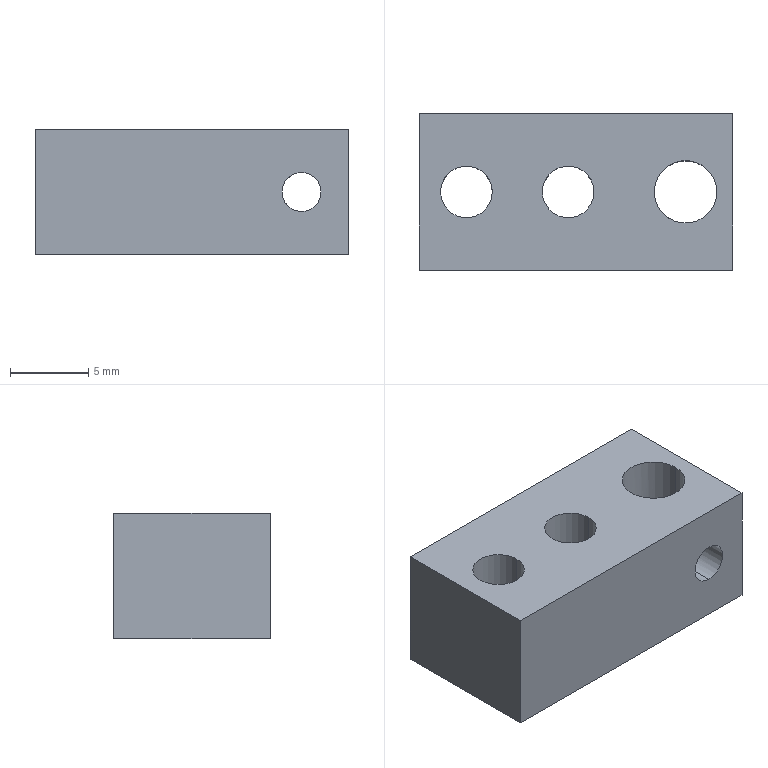Part | SolidWorks | features HoleWzd 2, Extrusion 1, ICE 1, MoveFace 1 | 1 solid | 16 faces | box 20 x 10 x 8 mm | volume 1332 mm3 | cylinder 10 | plane 6 | commonest cylinder face diameters 2.5 x4 3.3 x4 4 x2
STEP:
#1=CARTESIAN_POINT('',(0.,-5.,2.75));
#2=VERTEX_POINT('',#1);
#3=CARTESIAN_POINT('',(0.,-5.,5.25));
#4=VERTEX_POINT('',#3);
#5=CARTESIAN_POINT('',(0.,-5.,4.));
#6=DIRECTION('',(0.,1.,0.));
#7=DIRECTION('',(0.,0.,1.));
#8=AXIS2_PLACEMENT_3D('',#5,#6,#7);
#9=CIRCLE('',#8,1.25);
#10=EDGE_CURVE('',#2,#4,#9,.T.);
#11=ORIENTED_EDGE('',*,*,#10,.F.);
#12=CARTESIAN_POINT('',(0.,-2.,2.75));
#13=VERTEX_POINT('',#12);
#14=CARTESIAN_POINT('',(0.,5.,2.75));
#15=DIRECTION('',(0.,1.,0.));
#16=VECTOR('',#15,1000.);
#17=LINE('',#14,#16);
#18=EDGE_CURVE('',#2,#13,#17,.T.);
#19=ORIENTED_EDGE('',*,*,#18,.T.);
#20=CARTESIAN_POINT('',(0.,-2.,5.25));
#21=VERTEX_POINT('',#20);
#22=CARTESIAN_POINT('',(0.,-2.,2.75));
#23=CARTESIAN_POINT('',(-0.1686,-2.,2.75));
#24=CARTESIAN_POINT('',(-0.3364,-1.978,2.785));
#25=CARTESIAN_POINT('',(-0.6379,-1.902,2.913));
#26=CARTESIAN_POINT('',(-0.773,-1.849,3.005));
#27=CARTESIAN_POINT('',(-0.9982,-1.738,3.231));
#28=CARTESIAN_POINT('',(-1.088,-1.68,3.363));
#29=CARTESIAN_POINT('',(-1.183,-1.613,3.589));
#30=CARTESIAN_POINT('',(-1.208,-1.594,3.667));
#31=CARTESIAN_POINT('',(-1.241,-1.568,3.83));
#32=CARTESIAN_POINT('',(-1.25,-1.561,3.916));
#33=CARTESIAN_POINT('',(-1.25,-1.561,4.167));
#34=CARTESIAN_POINT('',(-1.215,-1.59,4.335));
#35=CARTESIAN_POINT('',(-1.089,-1.679,4.635));
#36=CARTESIAN_POINT('',(-0.9979,-1.738,4.769));
#37=CARTESIAN_POINT('',(-0.8293,-1.821,4.939));
#38=CARTESIAN_POINT('',(-0.7682,-1.848,4.989));
#39=CARTESIAN_POINT('',(-0.6354,-1.898,5.079));
#40=CARTESIAN_POINT('',(-0.5628,-1.921,5.119));
#41=CARTESIAN_POINT('',(-0.4124,-1.959,5.183));
#42=CARTESIAN_POINT('',(-0.3341,-1.974,5.207));
#43=CARTESIAN_POINT('',(-0.1706,-1.994,5.241));
#44=CARTESIAN_POINT('',(-0.08492,-2.,5.25));
#45=CARTESIAN_POINT('',(0.,-2.,5.25));
#46=B_SPLINE_CURVE_WITH_KNOTS('',3,(#22,#23,#24,#25,#26,#27,#28,#29,#30,#31,#32,#33,#34,#35,#36,#37,#38,#39,#40,#41,#42,#43,#44,#45),.UNSPECIFIED.,.F.,.F.,(4,2,2,2,2,2,2,2,2,2,2,4),(0.004021,0.004522,0.005024,0.005525,0.005776,0.006027,0.006528,0.00703,0.007281,0.007531,0.007782,0.008033),.UNSPECIFIED.);
#47=EDGE_CURVE('',#13,#21,#46,.T.);
#48=ORIENTED_EDGE('',*,*,#47,.T.);
#49=CARTESIAN_POINT('',(0.,5.,5.25));
#50=DIRECTION('',(0.,1.,0.));
#51=VECTOR('',#50,1000.);
#52=LINE('',#49,#51);
#53=EDGE_CURVE('',#4,#21,#52,.T.);
#54=ORIENTED_EDGE('',*,*,#53,.F.);
#55=EDGE_LOOP('',(#11,#19,#48,#54));
#56=FACE_OUTER_BOUND('',#55,.T.);
#57=CARTESIAN_POINT('',(0.,5.,4.));
#58=DIRECTION('',(0.,1.,0.));
#59=DIRECTION('',(0.,0.,1.));
#60=AXIS2_PLACEMENT_3D('',#57,#58,#59);
#61=CYLINDRICAL_SURFACE('',#60,1.25);
#62=ADVANCED_FACE('',(#56),#61,.F.);
#63=CARTESIAN_POINT('',(0.,2.,5.25));
#64=VERTEX_POINT('',#63);
#65=CARTESIAN_POINT('',(0.,2.,2.75));
#66=VERTEX_POINT('',#65);
#67=CARTESIAN_POINT('',(0.,2.,5.25));
#68=CARTESIAN_POINT('',(-0.08511,2.,5.25));
#69=CARTESIAN_POINT('',(-0.1684,1.995,5.241));
#70=CARTESIAN_POINT('',(-0.3316,1.974,5.208));
#71=CARTESIAN_POINT('',(-0.4122,1.959,5.183));
#72=CARTESIAN_POINT('',(-0.6385,1.902,5.087));
#73=CARTESIAN_POINT('',(-0.7738,1.848,4.994));
#74=CARTESIAN_POINT('',(-0.9977,1.738,4.77));
#75=CARTESIAN_POINT('',(-1.088,1.68,4.636));
#76=CARTESIAN_POINT('',(-1.214,1.591,4.338));
#77=CARTESIAN_POINT('',(-1.25,1.561,4.17));
#78=CARTESIAN_POINT('',(-1.25,1.561,3.831));
#79=CARTESIAN_POINT('',(-1.215,1.591,3.664));
#80=CARTESIAN_POINT('',(-1.089,1.68,3.365));
#81=CARTESIAN_POINT('',(-0.9982,1.738,3.231));
#82=CARTESIAN_POINT('',(-0.7723,1.849,3.004));
#83=CARTESIAN_POINT('',(-0.6398,1.901,2.913));
#84=CARTESIAN_POINT('',(-0.4108,1.959,2.817));
#85=CARTESIAN_POINT('',(-0.332,1.974,2.792));
#86=CARTESIAN_POINT('',(-0.1695,1.994,2.759));
#87=CARTESIAN_POINT('',(-0.0845,2.,2.75));
#88=CARTESIAN_POINT('',(0.,2.,2.75));
#89=B_SPLINE_CURVE_WITH_KNOTS('',3,(#67,#68,#69,#70,#71,#72,#73,#74,#75,#76,#77,#78,#79,#80,#81,#82,#83,#84,#85,#86,#87,#88),.UNSPECIFIED.,.F.,.F.,(4,2,2,2,2,2,2,2,2,2,4),(0.,0.0002513,0.0005026,0.001005,0.001508,0.002011,0.002513,0.003016,0.003518,0.00377,0.004021),.UNSPECIFIED.);
#90=EDGE_CURVE('',#64,#66,#89,.T.);
#91=ORIENTED_EDGE('',*,*,#90,.T.);
#92=CARTESIAN_POINT('',(0.,5.,2.75));
#93=VERTEX_POINT('',#92);
#94=CARTESIAN_POINT('',(0.,5.,2.75));
#95=DIRECTION('',(0.,1.,0.));
#96=VECTOR('',#95,1000.);
#97=LINE('',#94,#96);
#98=EDGE_CURVE('',#66,#93,#97,.T.);
#99=ORIENTED_EDGE('',*,*,#98,.T.);
#100=CARTESIAN_POINT('',(0.,5.,5.25));
#101=VERTEX_POINT('',#100);
#102=CARTESIAN_POINT('',(0.,5.,4.));
#103=DIRECTION('',(0.,1.,0.));
#104=DIRECTION('',(0.,0.,1.));
#105=AXIS2_PLACEMENT_3D('',#102,#103,#104);
#106=CIRCLE('',#105,1.25);
#107=EDGE_CURVE('',#93,#101,#106,.T.);
#108=ORIENTED_EDGE('',*,*,#107,.T.);
#109=CARTESIAN_POINT('',(0.,5.,5.25));
#110=DIRECTION('',(0.,1.,0.));
#111=VECTOR('',#110,1000.);
#112=LINE('',#109,#111);
#113=EDGE_CURVE('',#64,#101,#112,.T.);
#114=ORIENTED_EDGE('',*,*,#113,.F.);
#115=EDGE_LOOP('',(#91,#99,#108,#114));
#116=FACE_OUTER_BOUND('',#115,.T.);
#117=CARTESIAN_POINT('',(0.,5.,4.));
#118=DIRECTION('',(0.,1.,0.));
#119=DIRECTION('',(0.,0.,1.));
#120=AXIS2_PLACEMENT_3D('',#117,#118,#119);
#121=CYLINDRICAL_SURFACE('',#120,1.25);
#122=ADVANCED_FACE('',(#116),#121,.F.);
#123=CARTESIAN_POINT('',(-9.15,0.,8.));
#124=VERTEX_POINT('',#123);
#125=CARTESIAN_POINT('',(-5.85,0.,8.));
#126=VERTEX_POINT('',#125);
#127=CARTESIAN_POINT('',(-7.5,0.,8.));
#128=DIRECTION('',(0.,0.,1.));
#129=DIRECTION('',(1.,0.,0.));
#130=AXIS2_PLACEMENT_3D('',#127,#128,#129);
#131=CIRCLE('',#130,1.65);
#132=EDGE_CURVE('',#124,#126,#131,.T.);
#133=ORIENTED_EDGE('',*,*,#132,.T.);
#134=CARTESIAN_POINT('',(-5.85,0.,0.));
#135=VERTEX_POINT('',#134);
#136=CARTESIAN_POINT('',(-5.85,0.,0.));
#137=DIRECTION('',(0.,0.,-1.));
#138=VECTOR('',#137,1000.);
#139=LINE('',#136,#138);
#140=EDGE_CURVE('',#126,#135,#139,.T.);
#141=ORIENTED_EDGE('',*,*,#140,.T.);
#142=CARTESIAN_POINT('',(-9.15,0.,0.));
#143=VERTEX_POINT('',#142);
#144=CARTESIAN_POINT('',(-7.5,0.,0.));
#145=DIRECTION('',(0.,0.,-1.));
#146=DIRECTION('',(-1.,0.,0.));
#147=AXIS2_PLACEMENT_3D('',#144,#145,#146);
#148=CIRCLE('',#147,1.65);
#149=EDGE_CURVE('',#135,#143,#148,.T.);
#150=ORIENTED_EDGE('',*,*,#149,.T.);
#151=CARTESIAN_POINT('',(-9.15,0.,0.));
#152=DIRECTION('',(0.,0.,-1.));
#153=VECTOR('',#152,1000.);
#154=LINE('',#151,#153);
#155=EDGE_CURVE('',#124,#143,#154,.T.);
#156=ORIENTED_EDGE('',*,*,#155,.F.);
#157=EDGE_LOOP('',(#133,#141,#150,#156));
#158=FACE_OUTER_BOUND('',#157,.T.);
#159=CARTESIAN_POINT('',(-7.5,0.,0.));
#160=DIRECTION('',(0.,0.,-1.));
#161=DIRECTION('',(-1.,0.,0.));
#162=AXIS2_PLACEMENT_3D('',#159,#160,#161);
#163=CYLINDRICAL_SURFACE('',#162,1.65);
#164=ADVANCED_FACE('',(#158),#163,.F.);
#165=CARTESIAN_POINT('',(-15.65,0.,8.));
#166=VERTEX_POINT('',#165);
#167=CARTESIAN_POINT('',(-12.35,0.,8.));
#168=VERTEX_POINT('',#167);
#169=CARTESIAN_POINT('',(-14.,0.,8.));
#170=DIRECTION('',(0.,0.,1.));
#171=DIRECTION('',(1.,0.,0.));
#172=AXIS2_PLACEMENT_3D('',#169,#170,#171);
#173=CIRCLE('',#172,1.65);
#174=EDGE_CURVE('',#166,#168,#173,.T.);
#175=ORIENTED_EDGE('',*,*,#174,.T.);
#176=CARTESIAN_POINT('',(-12.35,0.,0.));
#177=VERTEX_POINT('',#176);
#178=CARTESIAN_POINT('',(-12.35,0.,0.));
#179=DIRECTION('',(0.,0.,-1.));
#180=VECTOR('',#179,1000.);
#181=LINE('',#178,#180);
#182=EDGE_CURVE('',#168,#177,#181,.T.);
#183=ORIENTED_EDGE('',*,*,#182,.T.);
#184=CARTESIAN_POINT('',(-15.65,0.,0.));
#185=VERTEX_POINT('',#184);
#186=CARTESIAN_POINT('',(-14.,0.,0.));
#187=DIRECTION('',(0.,0.,-1.));
#188=DIRECTION('',(-1.,0.,0.));
#189=AXIS2_PLACEMENT_3D('',#186,#187,#188);
#190=CIRCLE('',#189,1.65);
#191=EDGE_CURVE('',#177,#185,#190,.T.);
#192=ORIENTED_EDGE('',*,*,#191,.T.);
#193=CARTESIAN_POINT('',(-15.65,0.,0.));
#194=DIRECTION('',(0.,0.,-1.));
#195=VECTOR('',#194,1000.);
#196=LINE('',#193,#195);
#197=EDGE_CURVE('',#166,#185,#196,.T.);
#198=ORIENTED_EDGE('',*,*,#197,.F.);
#199=EDGE_LOOP('',(#175,#183,#192,#198));
#200=FACE_OUTER_BOUND('',#199,.T.);
#201=CARTESIAN_POINT('',(-14.,0.,0.));
#202=DIRECTION('',(0.,0.,-1.));
#203=DIRECTION('',(-1.,0.,0.));
#204=AXIS2_PLACEMENT_3D('',#201,#202,#203);
#205=CYLINDRICAL_SURFACE('',#204,1.65);
#206=ADVANCED_FACE('',(#200),#205,.F.);
#207=CARTESIAN_POINT('',(0.,-2.,5.25));
#208=CARTESIAN_POINT('',(0.08511,-2.,5.25));
#209=CARTESIAN_POINT('',(0.1684,-1.995,5.241));
#210=CARTESIAN_POINT('',(0.3316,-1.974,5.208));
#211=CARTESIAN_POINT('',(0.4122,-1.959,5.183));
#212=CARTESIAN_POINT('',(0.6385,-1.902,5.087));
#213=CARTESIAN_POINT('',(0.7738,-1.848,4.994));
#214=CARTESIAN_POINT('',(0.9977,-1.738,4.77));
#215=CARTESIAN_POINT('',(1.088,-1.68,4.636));
#216=CARTESIAN_POINT('',(1.214,-1.591,4.338));
#217=CARTESIAN_POINT('',(1.25,-1.561,4.17));
#218=CARTESIAN_POINT('',(1.25,-1.561,3.831));
#219=CARTESIAN_POINT('',(1.215,-1.591,3.664));
#220=CARTESIAN_POINT('',(1.089,-1.68,3.365));
#221=CARTESIAN_POINT('',(0.9982,-1.738,3.231));
#222=CARTESIAN_POINT('',(0.7723,-1.849,3.004));
#223=CARTESIAN_POINT('',(0.6398,-1.901,2.913));
#224=CARTESIAN_POINT('',(0.4108,-1.959,2.817));
#225=CARTESIAN_POINT('',(0.332,-1.974,2.792));
#226=CARTESIAN_POINT('',(0.1695,-1.994,2.759));
#227=CARTESIAN_POINT('',(0.0845,-2.,2.75));
#228=CARTESIAN_POINT('',(0.,-2.,2.75));
#229=B_SPLINE_CURVE_WITH_KNOTS('',3,(#207,#208,#209,#210,#211,#212,#213,#214,#215,#216,#217,#218,#219,#220,#221,#222,#223,#224,#225,#226,#227,#228),.UNSPECIFIED.,.F.,.F.,(4,2,2,2,2,2,2,2,2,2,4),(0.,0.0002513,0.0005026,0.001005,0.001508,0.002011,0.002513,0.003016,0.003518,0.00377,0.004021),.UNSPECIFIED.);
#230=EDGE_CURVE('',#21,#13,#229,.T.);
#231=ORIENTED_EDGE('',*,*,#230,.F.);
#232=ORIENTED_EDGE('',*,*,#47,.F.);
#233=EDGE_LOOP('',(#231,#232));
#234=FACE_BOUND('',#233,.T.);
#235=CARTESIAN_POINT('',(-2.,0.,8.));
#236=VERTEX_POINT('',#235);
#237=CARTESIAN_POINT('',(2.,0.,8.));
#238=VERTEX_POINT('',#237);
#239=CARTESIAN_POINT('',(0.,0.,8.));
#240=DIRECTION('',(0.,0.,1.));
#241=DIRECTION('',(1.,0.,0.));
#242=AXIS2_PLACEMENT_3D('',#239,#240,#241);
#243=CIRCLE('',#242,2.);
#244=EDGE_CURVE('',#236,#238,#243,.T.);
#245=ORIENTED_EDGE('',*,*,#244,.T.);
#246=CARTESIAN_POINT('',(2.,0.,0.));
#247=VERTEX_POINT('',#246);
#248=CARTESIAN_POINT('',(2.,0.,8.));
#249=DIRECTION('',(0.,0.,-1.));
#250=VECTOR('',#249,1000.);
#251=LINE('',#248,#250);
#252=EDGE_CURVE('',#238,#247,#251,.T.);
#253=ORIENTED_EDGE('',*,*,#252,.T.);
#254=CARTESIAN_POINT('',(-2.,0.,0.));
#255=VERTEX_POINT('',#254);
#256=CARTESIAN_POINT('',(0.,0.,0.));
#257=DIRECTION('',(0.,0.,1.));
#258=DIRECTION('',(1.,0.,0.));
#259=AXIS2_PLACEMENT_3D('',#256,#257,#258);
#260=CIRCLE('',#259,2.);
#261=EDGE_CURVE('',#255,#247,#260,.T.);
#262=ORIENTED_EDGE('',*,*,#261,.F.);
#263=CARTESIAN_POINT('',(-2.,0.,8.));
#264=DIRECTION('',(0.,0.,-1.));
#265=VECTOR('',#264,1000.);
#266=LINE('',#263,#265);
#267=EDGE_CURVE('',#236,#255,#266,.T.);
#268=ORIENTED_EDGE('',*,*,#267,.F.);
#269=EDGE_LOOP('',(#245,#253,#262,#268));
#270=FACE_OUTER_BOUND('',#269,.T.);
#271=CARTESIAN_POINT('',(0.,0.,8.));
#272=DIRECTION('',(0.,0.,-1.));
#273=DIRECTION('',(-1.,0.,0.));
#274=AXIS2_PLACEMENT_3D('',#271,#272,#273);
#275=CYLINDRICAL_SURFACE('',#274,2.);
#276=ADVANCED_FACE('',(#234,#270),#275,.F.);
#277=ORIENTED_EDGE('',*,*,#132,.F.);
#278=CARTESIAN_POINT('',(-7.5,0.,8.));
#279=DIRECTION('',(0.,0.,1.));
#280=DIRECTION('',(1.,0.,0.));
#281=AXIS2_PLACEMENT_3D('',#278,#279,#280);
#282=CIRCLE('',#281,1.65);
#283=EDGE_CURVE('',#126,#124,#282,.T.);
#284=ORIENTED_EDGE('',*,*,#283,.F.);
#285=EDGE_LOOP('',(#277,#284));
#286=FACE_BOUND('',#285,.T.);
#287=ORIENTED_EDGE('',*,*,#174,.F.);
#288=CARTESIAN_POINT('',(-14.,0.,8.));
#289=DIRECTION('',(0.,0.,1.));
#290=DIRECTION('',(1.,0.,0.));
#291=AXIS2_PLACEMENT_3D('',#288,#289,#290);
#292=CIRCLE('',#291,1.65);
#293=EDGE_CURVE('',#168,#166,#292,.T.);
#294=ORIENTED_EDGE('',*,*,#293,.F.);
#295=EDGE_LOOP('',(#287,#294));
#296=FACE_BOUND('',#295,.T.);
#297=CARTESIAN_POINT('',(3.,5.,8.));
#298=VERTEX_POINT('',#297);
#299=CARTESIAN_POINT('',(3.,-5.,8.));
#300=VERTEX_POINT('',#299);
#301=CARTESIAN_POINT('',(3.,0.,8.));
#302=DIRECTION('',(0.,-1.,0.));
#303=VECTOR('',#302,1000.);
#304=LINE('',#301,#303);
#305=EDGE_CURVE('',#298,#300,#304,.T.);
#306=ORIENTED_EDGE('',*,*,#305,.F.);
#307=CARTESIAN_POINT('',(-17.,5.,8.));
#308=VERTEX_POINT('',#307);
#309=CARTESIAN_POINT('',(-10.,5.,8.));
#310=DIRECTION('',(-1.,0.,0.));
#311=VECTOR('',#310,1000.);
#312=LINE('',#309,#311);
#313=EDGE_CURVE('',#298,#308,#312,.T.);
#314=ORIENTED_EDGE('',*,*,#313,.T.);
#315=CARTESIAN_POINT('',(-17.,-5.,8.));
#316=VERTEX_POINT('',#315);
#317=CARTESIAN_POINT('',(-17.,5.,8.));
#318=DIRECTION('',(0.,-1.,0.));
#319=VECTOR('',#318,1000.);
#320=LINE('',#317,#319);
#321=EDGE_CURVE('',#308,#316,#320,.T.);
#322=ORIENTED_EDGE('',*,*,#321,.T.);
#323=CARTESIAN_POINT('',(-10.,-5.,8.));
#324=DIRECTION('',(1.,0.,0.));
#325=VECTOR('',#324,1000.);
#326=LINE('',#323,#325);
#327=EDGE_CURVE('',#316,#300,#326,.T.);
#328=ORIENTED_EDGE('',*,*,#327,.T.);
#329=EDGE_LOOP('',(#306,#314,#322,#328));
#330=FACE_OUTER_BOUND('',#329,.T.);
#331=ORIENTED_EDGE('',*,*,#244,.F.);
#332=CARTESIAN_POINT('',(0.,0.,8.));
#333=DIRECTION('',(0.,0.,1.));
#334=DIRECTION('',(1.,0.,0.));
#335=AXIS2_PLACEMENT_3D('',#332,#333,#334);
#336=CIRCLE('',#335,2.);
#337=EDGE_CURVE('',#238,#236,#336,.T.);
#338=ORIENTED_EDGE('',*,*,#337,.F.);
#339=EDGE_LOOP('',(#331,#338));
#340=FACE_BOUND('',#339,.T.);
#341=CARTESIAN_POINT('',(0.,0.,8.));
#342=DIRECTION('',(0.,0.,1.));
#343=DIRECTION('',(1.,0.,0.));
#344=AXIS2_PLACEMENT_3D('',#341,#342,#343);
#345=PLANE('',#344);
#346=ADVANCED_FACE('',(#286,#296,#330,#340),#345,.T.);
#347=CARTESIAN_POINT('',(-7.5,0.,0.));
#348=DIRECTION('',(0.,0.,-1.));
#349=DIRECTION('',(-1.,0.,0.));
#350=AXIS2_PLACEMENT_3D('',#347,#348,#349);
#351=CIRCLE('',#350,1.65);
#352=EDGE_CURVE('',#143,#135,#351,.T.);
#353=ORIENTED_EDGE('',*,*,#352,.F.);
#354=ORIENTED_EDGE('',*,*,#149,.F.);
#355=EDGE_LOOP('',(#353,#354));
#356=FACE_BOUND('',#355,.T.);
#357=CARTESIAN_POINT('',(-14.,0.,0.));
#358=DIRECTION('',(0.,0.,-1.));
#359=DIRECTION('',(-1.,0.,0.));
#360=AXIS2_PLACEMENT_3D('',#357,#358,#359);
#361=CIRCLE('',#360,1.65);
#362=EDGE_CURVE('',#185,#177,#361,.T.);
#363=ORIENTED_EDGE('',*,*,#362,.F.);
#364=ORIENTED_EDGE('',*,*,#191,.F.);
#365=EDGE_LOOP('',(#363,#364));
#366=FACE_BOUND('',#365,.T.);
#367=CARTESIAN_POINT('',(3.,5.,0.));
#368=VERTEX_POINT('',#367);
#369=CARTESIAN_POINT('',(-17.,5.,0.));
#370=VERTEX_POINT('',#369);
#371=CARTESIAN_POINT('',(-10.,5.,0.));
#372=DIRECTION('',(-1.,0.,0.));
#373=VECTOR('',#372,1000.);
#374=LINE('',#371,#373);
#375=EDGE_CURVE('',#368,#370,#374,.T.);
#376=ORIENTED_EDGE('',*,*,#375,.F.);
#377=CARTESIAN_POINT('',(3.,-5.,0.));
#378=VERTEX_POINT('',#377);
#379=CARTESIAN_POINT('',(3.,10.325,0.));
#380=DIRECTION('',(0.,1.,0.));
#381=VECTOR('',#380,1000.);
#382=LINE('',#379,#381);
#383=EDGE_CURVE('',#378,#368,#382,.T.);
#384=ORIENTED_EDGE('',*,*,#383,.F.);
#385=CARTESIAN_POINT('',(-17.,-5.,0.));
#386=VERTEX_POINT('',#385);
#387=CARTESIAN_POINT('',(-10.,-5.,0.));
#388=DIRECTION('',(1.,0.,0.));
#389=VECTOR('',#388,1000.);
#390=LINE('',#387,#389);
#391=EDGE_CURVE('',#386,#378,#390,.T.);
#392=ORIENTED_EDGE('',*,*,#391,.F.);
#393=CARTESIAN_POINT('',(-17.,5.,0.));
#394=DIRECTION('',(0.,-1.,0.));
#395=VECTOR('',#394,1000.);
#396=LINE('',#393,#395);
#397=EDGE_CURVE('',#370,#386,#396,.T.);
#398=ORIENTED_EDGE('',*,*,#397,.F.);
#399=EDGE_LOOP('',(#376,#384,#392,#398));
#400=FACE_OUTER_BOUND('',#399,.T.);
#401=ORIENTED_EDGE('',*,*,#261,.T.);
#402=CARTESIAN_POINT('',(0.,0.,0.));
#403=DIRECTION('',(0.,0.,1.));
#404=DIRECTION('',(1.,0.,0.));
#405=AXIS2_PLACEMENT_3D('',#402,#403,#404);
#406=CIRCLE('',#405,2.);
#407=EDGE_CURVE('',#247,#255,#406,.T.);
#408=ORIENTED_EDGE('',*,*,#407,.T.);
#409=EDGE_LOOP('',(#401,#408));
#410=FACE_BOUND('',#409,.T.);
#411=CARTESIAN_POINT('',(0.,0.,0.));
#412=DIRECTION('',(0.,0.,1.));
#413=DIRECTION('',(1.,0.,0.));
#414=AXIS2_PLACEMENT_3D('',#411,#412,#413);
#415=PLANE('',#414);
#416=ADVANCED_FACE('',(#356,#366,#400,#410),#415,.F.);
#417=CARTESIAN_POINT('',(0.,5.,4.));
#418=DIRECTION('',(0.,1.,0.));
#419=DIRECTION('',(0.,0.,1.));
#420=AXIS2_PLACEMENT_3D('',#417,#418,#419);
#421=CIRCLE('',#420,1.25);
#422=EDGE_CURVE('',#101,#93,#421,.T.);
#423=ORIENTED_EDGE('',*,*,#422,.F.);
#424=ORIENTED_EDGE('',*,*,#107,.F.);
#425=EDGE_LOOP('',(#423,#424));
#426=FACE_BOUND('',#425,.T.);
#427=ORIENTED_EDGE('',*,*,#313,.F.);
#428=CARTESIAN_POINT('',(3.,5.,8.));
#429=DIRECTION('',(0.,0.,-1.));
#430=VECTOR('',#429,1000.);
#431=LINE('',#428,#430);
#432=EDGE_CURVE('',#298,#368,#431,.T.);
#433=ORIENTED_EDGE('',*,*,#432,.T.);
#434=ORIENTED_EDGE('',*,*,#375,.T.);
#435=CARTESIAN_POINT('',(-17.,5.,8.));
#436=DIRECTION('',(0.,0.,-1.));
#437=VECTOR('',#436,1000.);
#438=LINE('',#435,#437);
#439=EDGE_CURVE('',#308,#370,#438,.T.);
#440=ORIENTED_EDGE('',*,*,#439,.F.);
#441=EDGE_LOOP('',(#427,#433,#434,#440));
#442=FACE_OUTER_BOUND('',#441,.T.);
#443=CARTESIAN_POINT('',(-10.,5.,8.));
#444=DIRECTION('',(0.,-1.,0.));
#445=DIRECTION('',(0.,0.,-1.));
#446=AXIS2_PLACEMENT_3D('',#443,#444,#445);
#447=PLANE('',#446);
#448=ADVANCED_FACE('',(#426,#442),#447,.F.);
#449=ORIENTED_EDGE('',*,*,#397,.T.);
#450=CARTESIAN_POINT('',(-17.,-5.,8.));
#451=DIRECTION('',(0.,0.,-1.));
#452=VECTOR('',#451,1000.);
#453=LINE('',#450,#452);
#454=EDGE_CURVE('',#316,#386,#453,.T.);
#455=ORIENTED_EDGE('',*,*,#454,.F.);
#456=ORIENTED_EDGE('',*,*,#321,.F.);
#457=ORIENTED_EDGE('',*,*,#439,.T.);
#458=EDGE_LOOP('',(#449,#455,#456,#457));
#459=FACE_OUTER_BOUND('',#458,.T.);
#460=CARTESIAN_POINT('',(-17.,5.,8.));
#461=DIRECTION('',(1.,0.,0.));
#462=DIRECTION('',(0.,1.,0.));
#463=AXIS2_PLACEMENT_3D('',#460,#461,#462);
#464=PLANE('',#463);
#465=ADVANCED_FACE('',(#459),#464,.F.);
#466=CARTESIAN_POINT('',(0.,-5.,4.));
#467=DIRECTION('',(0.,1.,0.));
#468=DIRECTION('',(0.,0.,1.));
#469=AXIS2_PLACEMENT_3D('',#466,#467,#468);
#470=CIRCLE('',#469,1.25);
#471=EDGE_CURVE('',#4,#2,#470,.T.);
#472=ORIENTED_EDGE('',*,*,#471,.T.);
#473=ORIENTED_EDGE('',*,*,#10,.T.);
#474=EDGE_LOOP('',(#472,#473));
#475=FACE_BOUND('',#474,.T.);
#476=ORIENTED_EDGE('',*,*,#391,.T.);
#477=CARTESIAN_POINT('',(3.,-5.,8.));
#478=DIRECTION('',(0.,0.,1.));
#479=VECTOR('',#478,1000.);
#480=LINE('',#477,#479);
#481=EDGE_CURVE('',#378,#300,#480,.T.);
#482=ORIENTED_EDGE('',*,*,#481,.T.);
#483=ORIENTED_EDGE('',*,*,#327,.F.);
#484=ORIENTED_EDGE('',*,*,#454,.T.);
#485=EDGE_LOOP('',(#476,#482,#483,#484));
#486=FACE_OUTER_BOUND('',#485,.T.);
#487=CARTESIAN_POINT('',(-10.,-5.,8.));
#488=DIRECTION('',(0.,1.,0.));
#489=DIRECTION('',(0.,0.,1.));
#490=AXIS2_PLACEMENT_3D('',#487,#488,#489);
#491=PLANE('',#490);
#492=ADVANCED_FACE('',(#475,#486),#491,.F.);
#493=ORIENTED_EDGE('',*,*,#252,.F.);
#494=ORIENTED_EDGE('',*,*,#337,.T.);
#495=ORIENTED_EDGE('',*,*,#267,.T.);
#496=ORIENTED_EDGE('',*,*,#407,.F.);
#497=EDGE_LOOP('',(#493,#494,#495,#496));
#498=FACE_OUTER_BOUND('',#497,.T.);
#499=ORIENTED_EDGE('',*,*,#90,.F.);
#500=CARTESIAN_POINT('',(0.,2.,2.75));
#501=CARTESIAN_POINT('',(0.1686,2.,2.75));
#502=CARTESIAN_POINT('',(0.3364,1.978,2.785));
#503=CARTESIAN_POINT('',(0.6379,1.902,2.913));
#504=CARTESIAN_POINT('',(0.773,1.849,3.005));
#505=CARTESIAN_POINT('',(0.9982,1.738,3.231));
#506=CARTESIAN_POINT('',(1.088,1.68,3.363));
#507=CARTESIAN_POINT('',(1.183,1.613,3.589));
#508=CARTESIAN_POINT('',(1.208,1.594,3.667));
#509=CARTESIAN_POINT('',(1.241,1.568,3.83));
#510=CARTESIAN_POINT('',(1.25,1.561,3.916));
#511=CARTESIAN_POINT('',(1.25,1.561,4.167));
#512=CARTESIAN_POINT('',(1.215,1.59,4.335));
#513=CARTESIAN_POINT('',(1.089,1.679,4.635));
#514=CARTESIAN_POINT('',(0.9979,1.738,4.769));
#515=CARTESIAN_POINT('',(0.8293,1.821,4.939));
#516=CARTESIAN_POINT('',(0.7682,1.848,4.989));
#517=CARTESIAN_POINT('',(0.6354,1.898,5.079));
#518=CARTESIAN_POINT('',(0.5628,1.921,5.119));
#519=CARTESIAN_POINT('',(0.4124,1.959,5.183));
#520=CARTESIAN_POINT('',(0.3341,1.974,5.207));
#521=CARTESIAN_POINT('',(0.1706,1.994,5.241));
#522=CARTESIAN_POINT('',(0.08492,2.,5.25));
#523=CARTESIAN_POINT('',(0.,2.,5.25));
#524=B_SPLINE_CURVE_WITH_KNOTS('',3,(#500,#501,#502,#503,#504,#505,#506,#507,#508,#509,#510,#511,#512,#513,#514,#515,#516,#517,#518,#519,#520,#521,#522,#523),.UNSPECIFIED.,.F.,.F.,(4,2,2,2,2,2,2,2,2,2,2,4),(0.004021,0.004522,0.005024,0.005525,0.005776,0.006027,0.006528,0.00703,0.007281,0.007531,0.007782,0.008033),.UNSPECIFIED.);
#525=EDGE_CURVE('',#66,#64,#524,.T.);
#526=ORIENTED_EDGE('',*,*,#525,.F.);
#527=EDGE_LOOP('',(#499,#526));
#528=FACE_BOUND('',#527,.T.);
#529=CARTESIAN_POINT('',(0.,0.,8.));
#530=DIRECTION('',(0.,0.,-1.));
#531=DIRECTION('',(-1.,0.,0.));
#532=AXIS2_PLACEMENT_3D('',#529,#530,#531);
#533=CYLINDRICAL_SURFACE('',#532,2.);
#534=ADVANCED_FACE('',(#498,#528),#533,.F.);
#535=ORIENTED_EDGE('',*,*,#305,.T.);
#536=ORIENTED_EDGE('',*,*,#481,.F.);
#537=ORIENTED_EDGE('',*,*,#383,.T.);
#538=ORIENTED_EDGE('',*,*,#432,.F.);
#539=EDGE_LOOP('',(#535,#536,#537,#538));
#540=FACE_OUTER_BOUND('',#539,.T.);
#541=CARTESIAN_POINT('',(3.,10.325,22.));
#542=DIRECTION('',(-1.,0.,0.));
#543=DIRECTION('',(0.,-1.,0.));
#544=AXIS2_PLACEMENT_3D('',#541,#542,#543);
#545=PLANE('',#544);
#546=ADVANCED_FACE('',(#540),#545,.F.);
#547=ORIENTED_EDGE('',*,*,#182,.F.);
#548=ORIENTED_EDGE('',*,*,#293,.T.);
#549=ORIENTED_EDGE('',*,*,#197,.T.);
#550=ORIENTED_EDGE('',*,*,#362,.T.);
#551=EDGE_LOOP('',(#547,#548,#549,#550));
#552=FACE_OUTER_BOUND('',#551,.T.);
#553=CARTESIAN_POINT('',(-14.,0.,0.));
#554=DIRECTION('',(0.,0.,-1.));
#555=DIRECTION('',(-1.,0.,0.));
#556=AXIS2_PLACEMENT_3D('',#553,#554,#555);
#557=CYLINDRICAL_SURFACE('',#556,1.65);
#558=ADVANCED_FACE('',(#552),#557,.F.);
#559=ORIENTED_EDGE('',*,*,#140,.F.);
#560=ORIENTED_EDGE('',*,*,#283,.T.);
#561=ORIENTED_EDGE('',*,*,#155,.T.);
#562=ORIENTED_EDGE('',*,*,#352,.T.);
#563=EDGE_LOOP('',(#559,#560,#561,#562));
#564=FACE_OUTER_BOUND('',#563,.T.);
#565=CARTESIAN_POINT('',(-7.5,0.,0.));
#566=DIRECTION('',(0.,0.,-1.));
#567=DIRECTION('',(-1.,0.,0.));
#568=AXIS2_PLACEMENT_3D('',#565,#566,#567);
#569=CYLINDRICAL_SURFACE('',#568,1.65);
#570=ADVANCED_FACE('',(#564),#569,.F.);
#571=ORIENTED_EDGE('',*,*,#98,.F.);
#572=ORIENTED_EDGE('',*,*,#525,.T.);
#573=ORIENTED_EDGE('',*,*,#113,.T.);
#574=ORIENTED_EDGE('',*,*,#422,.T.);
#575=EDGE_LOOP('',(#571,#572,#573,#574));
#576=FACE_OUTER_BOUND('',#575,.T.);
#577=CARTESIAN_POINT('',(0.,5.,4.));
#578=DIRECTION('',(0.,1.,0.));
#579=DIRECTION('',(0.,0.,1.));
#580=AXIS2_PLACEMENT_3D('',#577,#578,#579);
#581=CYLINDRICAL_SURFACE('',#580,1.25);
#582=ADVANCED_FACE('',(#576),#581,.F.);
#583=ORIENTED_EDGE('',*,*,#18,.F.);
#584=ORIENTED_EDGE('',*,*,#471,.F.);
#585=ORIENTED_EDGE('',*,*,#53,.T.);
#586=ORIENTED_EDGE('',*,*,#230,.T.);
#587=EDGE_LOOP('',(#583,#584,#585,#586));
#588=FACE_OUTER_BOUND('',#587,.T.);
#589=CARTESIAN_POINT('',(0.,5.,4.));
#590=DIRECTION('',(0.,1.,0.));
#591=DIRECTION('',(0.,0.,1.));
#592=AXIS2_PLACEMENT_3D('',#589,#590,#591);
#593=CYLINDRICAL_SURFACE('',#592,1.25);
#594=ADVANCED_FACE('',(#588),#593,.F.);
#595=CLOSED_SHELL('',(#62,#122,#164,#206,#276,#346,#416,#448,#465,#492,#534,#546,#558,#570,#582,#594));
#596=MANIFOLD_SOLID_BREP('',#595);
#597=CARTESIAN_POINT('',(0.,0.,0.));
#598=DIRECTION('',(0.,0.,1.));
#599=DIRECTION('',(1.,0.,0.));
#600=AXIS2_PLACEMENT_3D('',#597,#598,#599);
#601=(LENGTH_UNIT()NAMED_UNIT(*)SI_UNIT(.MILLI.,.METRE.));
#602=UNCERTAINTY_MEASURE_WITH_UNIT(LENGTH_MEASURE(0.00001),#601,'','');
#603=(NAMED_UNIT(*)PLANE_ANGLE_UNIT()SI_UNIT($,.RADIAN.));
#604=(NAMED_UNIT(*)SI_UNIT($,.STERADIAN.)SOLID_ANGLE_UNIT());
#605=(GEOMETRIC_REPRESENTATION_CONTEXT(3)GLOBAL_UNCERTAINTY_ASSIGNED_CONTEXT((#602))GLOBAL_UNIT_ASSIGNED_CONTEXT((#601,#603,#604))REPRESENTATION_CONTEXT('',''));
#606=ADVANCED_BREP_SHAPE_REPRESENTATION('',(#596,#600),#605);